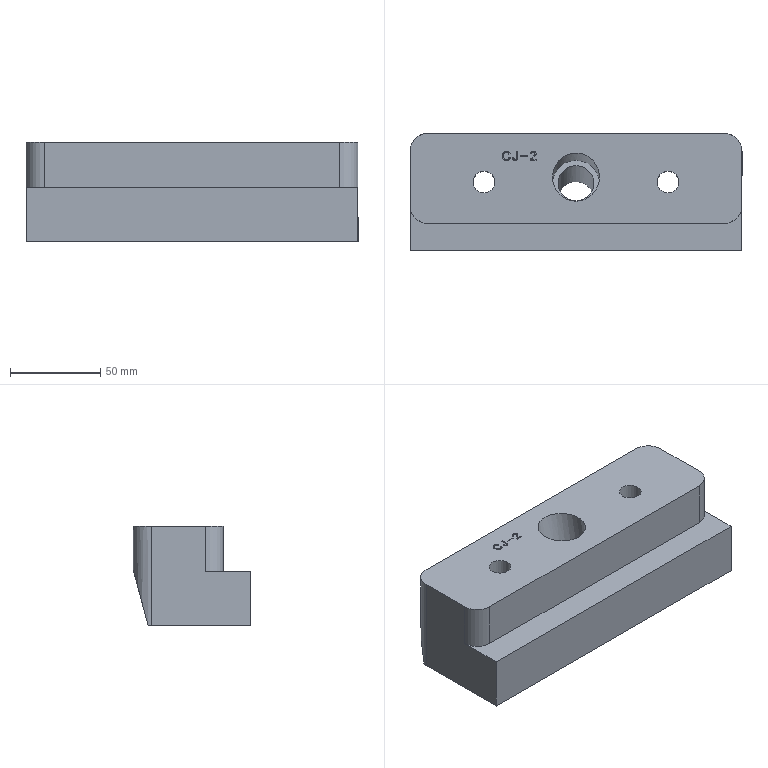Part | STEP file | solid 18 | 1 solid | 46 faces | box 184 x 65 x 55 mm | volume 526326 mm3 | plane 30 | cylinder 10 | other 6 | commonest cylinder face diameters 20 x5 12 x2 18 x2 26 x1